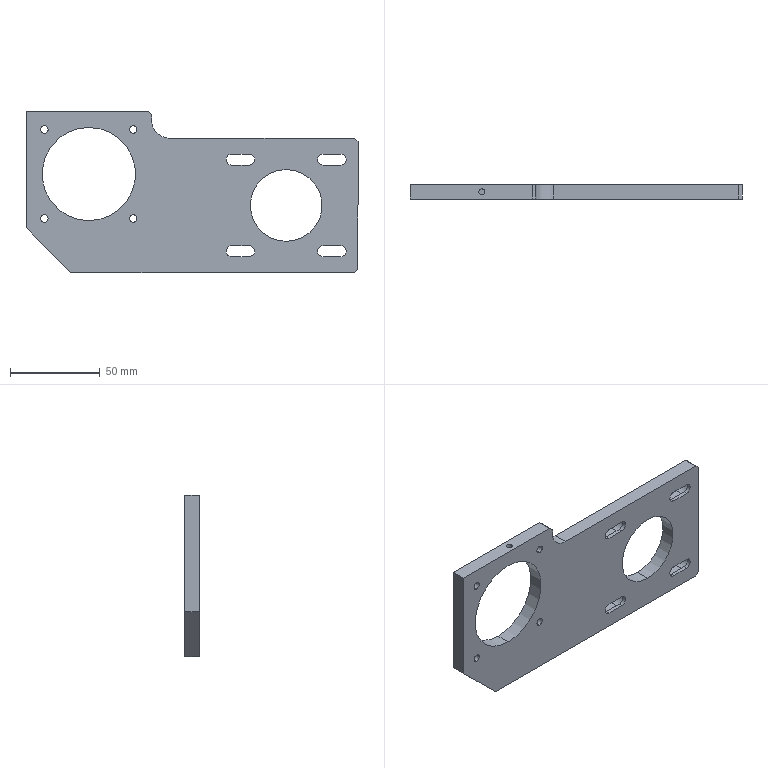Part | SolidWorks | features ICE 5, HoleWzd 3, Chamfer 2, Extrusion 1, Fillet 1 | 1 solid | 71 faces | box 185 x 8 x 90 mm | volume 84254 mm3 | cylinder 35 | plane 32 | cone 4 | commonest cylinder face diameters 4.2 x8 6 x8 10 x8 3.3 x6 40 x2 52 x2